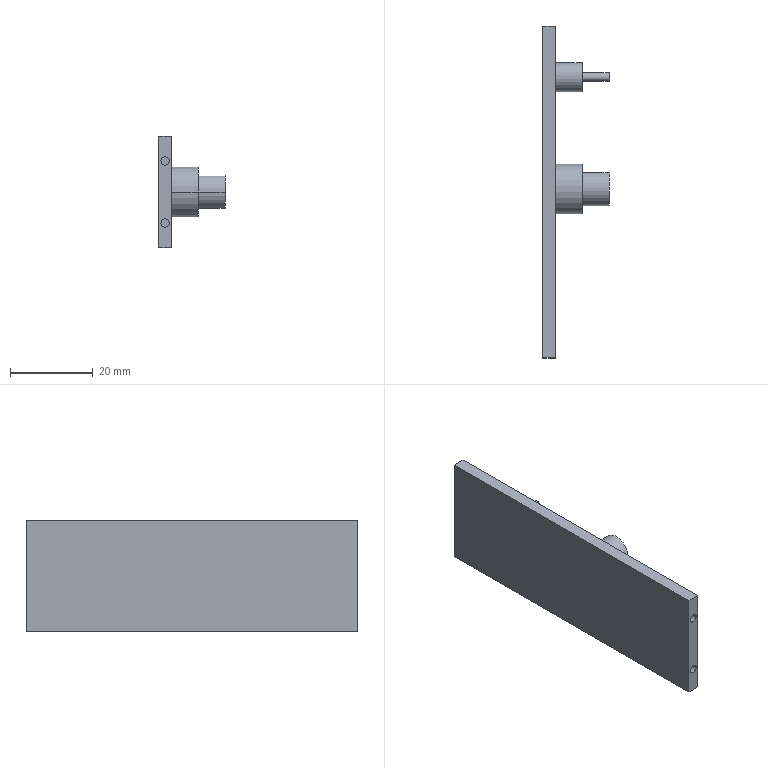Part | SolidWorks | features ICE 2, Cut 1, Extrusion 1 | 1 solid | 24 faces | box 16 x 80 x 27 mm | volume 7781 mm3 | cylinder 12 | plane 12 | commonest cylinder face diameters 2 x6 7 x2 8 x2 12 x2
STEP:
#1=CARTESIAN_POINT('',(-0.4828,4.071,21.));
#2=VERTEX_POINT('',#1);
#3=CARTESIAN_POINT('',(1.517,4.071,21.));
#4=VERTEX_POINT('',#3);
#5=CARTESIAN_POINT('',(0.5172,4.071,21.));
#6=DIRECTION('',(0.,-1.,0.));
#7=DIRECTION('',(1.,0.,0.));
#8=AXIS2_PLACEMENT_3D('',#5,#6,#7);
#9=CIRCLE('',#8,1.);
#10=EDGE_CURVE('',#2,#4,#9,.T.);
#11=ORIENTED_EDGE('',*,*,#10,.F.);
#12=CARTESIAN_POINT('',(-0.4828,-0.9287,21.));
#13=VERTEX_POINT('',#12);
#14=CARTESIAN_POINT('',(-0.4828,4.071,21.));
#15=DIRECTION('',(0.,-1.,0.));
#16=VECTOR('',#15,1000.);
#17=LINE('',#14,#16);
#18=EDGE_CURVE('',#2,#13,#17,.T.);
#19=ORIENTED_EDGE('',*,*,#18,.T.);
#20=CARTESIAN_POINT('',(1.517,-0.9287,21.));
#21=VERTEX_POINT('',#20);
#22=CARTESIAN_POINT('',(0.5172,-0.9287,21.));
#23=DIRECTION('',(0.,1.,0.));
#24=DIRECTION('',(0.,0.,1.));
#25=AXIS2_PLACEMENT_3D('',#22,#23,#24);
#26=CIRCLE('',#25,1.);
#27=EDGE_CURVE('',#21,#13,#26,.T.);
#28=ORIENTED_EDGE('',*,*,#27,.F.);
#29=CARTESIAN_POINT('',(1.517,4.071,21.));
#30=DIRECTION('',(0.,-1.,0.));
#31=VECTOR('',#30,1000.);
#32=LINE('',#29,#31);
#33=EDGE_CURVE('',#4,#21,#32,.T.);
#34=ORIENTED_EDGE('',*,*,#33,.F.);
#35=EDGE_LOOP('',(#11,#19,#28,#34));
#36=FACE_OUTER_BOUND('',#35,.T.);
#37=CARTESIAN_POINT('',(0.5172,4.071,21.));
#38=DIRECTION('',(0.,-1.,0.));
#39=DIRECTION('',(1.,0.,0.));
#40=AXIS2_PLACEMENT_3D('',#37,#38,#39);
#41=CYLINDRICAL_SURFACE('',#40,1.);
#42=ADVANCED_FACE('',(#36),#41,.F.);
#43=CARTESIAN_POINT('',(-0.4828,4.071,6.));
#44=VERTEX_POINT('',#43);
#45=CARTESIAN_POINT('',(1.517,4.071,6.));
#46=VERTEX_POINT('',#45);
#47=CARTESIAN_POINT('',(0.5172,4.071,6.));
#48=DIRECTION('',(0.,-1.,0.));
#49=DIRECTION('',(1.,0.,0.));
#50=AXIS2_PLACEMENT_3D('',#47,#48,#49);
#51=CIRCLE('',#50,1.);
#52=EDGE_CURVE('',#44,#46,#51,.T.);
#53=ORIENTED_EDGE('',*,*,#52,.F.);
#54=CARTESIAN_POINT('',(-0.4828,-0.9287,6.));
#55=VERTEX_POINT('',#54);
#56=CARTESIAN_POINT('',(-0.4828,4.071,6.));
#57=DIRECTION('',(0.,-1.,0.));
#58=VECTOR('',#57,1000.);
#59=LINE('',#56,#58);
#60=EDGE_CURVE('',#44,#55,#59,.T.);
#61=ORIENTED_EDGE('',*,*,#60,.T.);
#62=CARTESIAN_POINT('',(1.517,-0.9287,6.));
#63=VERTEX_POINT('',#62);
#64=CARTESIAN_POINT('',(0.5172,-0.9287,6.));
#65=DIRECTION('',(0.,1.,0.));
#66=DIRECTION('',(0.,0.,1.));
#67=AXIS2_PLACEMENT_3D('',#64,#65,#66);
#68=CIRCLE('',#67,1.);
#69=EDGE_CURVE('',#63,#55,#68,.T.);
#70=ORIENTED_EDGE('',*,*,#69,.F.);
#71=CARTESIAN_POINT('',(1.517,4.071,6.));
#72=DIRECTION('',(0.,-1.,0.));
#73=VECTOR('',#72,1000.);
#74=LINE('',#71,#73);
#75=EDGE_CURVE('',#46,#63,#74,.T.);
#76=ORIENTED_EDGE('',*,*,#75,.F.);
#77=EDGE_LOOP('',(#53,#61,#70,#76));
#78=FACE_OUTER_BOUND('',#77,.T.);
#79=CARTESIAN_POINT('',(0.5172,4.071,6.));
#80=DIRECTION('',(0.,-1.,0.));
#81=DIRECTION('',(1.,0.,0.));
#82=AXIS2_PLACEMENT_3D('',#79,#80,#81);
#83=CYLINDRICAL_SURFACE('',#82,1.);
#84=ADVANCED_FACE('',(#78),#83,.F.);
#85=CARTESIAN_POINT('',(15.017,43.771,13.5));
#86=VERTEX_POINT('',#85);
#87=CARTESIAN_POINT('',(15.017,35.771,13.5));
#88=VERTEX_POINT('',#87);
#89=CARTESIAN_POINT('',(15.017,39.771,13.5));
#90=DIRECTION('',(1.,0.,0.));
#91=DIRECTION('',(0.,1.,0.));
#92=AXIS2_PLACEMENT_3D('',#89,#90,#91);
#93=CIRCLE('',#92,4.);
#94=EDGE_CURVE('',#86,#88,#93,.T.);
#95=ORIENTED_EDGE('',*,*,#94,.F.);
#96=CARTESIAN_POINT('',(8.517,43.771,13.5));
#97=VERTEX_POINT('',#96);
#98=CARTESIAN_POINT('',(15.017,43.771,13.5));
#99=DIRECTION('',(-1.,0.,0.));
#100=VECTOR('',#99,1000.);
#101=LINE('',#98,#100);
#102=EDGE_CURVE('',#86,#97,#101,.T.);
#103=ORIENTED_EDGE('',*,*,#102,.T.);
#104=CARTESIAN_POINT('',(8.517,35.771,13.5));
#105=VERTEX_POINT('',#104);
#106=CARTESIAN_POINT('',(8.517,39.771,13.5));
#107=DIRECTION('',(1.,0.,0.));
#108=DIRECTION('',(0.,1.,0.));
#109=AXIS2_PLACEMENT_3D('',#106,#107,#108);
#110=CIRCLE('',#109,4.);
#111=EDGE_CURVE('',#97,#105,#110,.T.);
#112=ORIENTED_EDGE('',*,*,#111,.T.);
#113=CARTESIAN_POINT('',(15.017,35.771,13.5));
#114=DIRECTION('',(-1.,0.,0.));
#115=VECTOR('',#114,1000.);
#116=LINE('',#113,#115);
#117=EDGE_CURVE('',#88,#105,#116,.T.);
#118=ORIENTED_EDGE('',*,*,#117,.F.);
#119=EDGE_LOOP('',(#95,#103,#112,#118));
#120=FACE_OUTER_BOUND('',#119,.T.);
#121=CARTESIAN_POINT('',(15.017,39.771,13.5));
#122=DIRECTION('',(-1.,0.,0.));
#123=DIRECTION('',(0.,-1.,0.));
#124=AXIS2_PLACEMENT_3D('',#121,#122,#123);
#125=CYLINDRICAL_SURFACE('',#124,4.);
#126=ADVANCED_FACE('',(#120),#125,.T.);
#127=CARTESIAN_POINT('',(15.017,67.771,13.5));
#128=VERTEX_POINT('',#127);
#129=CARTESIAN_POINT('',(15.017,65.771,13.5));
#130=VERTEX_POINT('',#129);
#131=CARTESIAN_POINT('',(15.017,66.771,13.5));
#132=DIRECTION('',(1.,0.,0.));
#133=DIRECTION('',(0.,1.,0.));
#134=AXIS2_PLACEMENT_3D('',#131,#132,#133);
#135=CIRCLE('',#134,1.);
#136=EDGE_CURVE('',#128,#130,#135,.T.);
#137=ORIENTED_EDGE('',*,*,#136,.F.);
#138=CARTESIAN_POINT('',(8.517,67.771,13.5));
#139=VERTEX_POINT('',#138);
#140=CARTESIAN_POINT('',(15.017,67.771,13.5));
#141=DIRECTION('',(-1.,0.,0.));
#142=VECTOR('',#141,1000.);
#143=LINE('',#140,#142);
#144=EDGE_CURVE('',#128,#139,#143,.T.);
#145=ORIENTED_EDGE('',*,*,#144,.T.);
#146=CARTESIAN_POINT('',(8.517,65.771,13.5));
#147=VERTEX_POINT('',#146);
#148=CARTESIAN_POINT('',(8.517,66.771,13.5));
#149=DIRECTION('',(1.,0.,0.));
#150=DIRECTION('',(0.,1.,0.));
#151=AXIS2_PLACEMENT_3D('',#148,#149,#150);
#152=CIRCLE('',#151,1.);
#153=EDGE_CURVE('',#139,#147,#152,.T.);
#154=ORIENTED_EDGE('',*,*,#153,.T.);
#155=CARTESIAN_POINT('',(15.017,65.771,13.5));
#156=DIRECTION('',(-1.,0.,0.));
#157=VECTOR('',#156,1000.);
#158=LINE('',#155,#157);
#159=EDGE_CURVE('',#130,#147,#158,.T.);
#160=ORIENTED_EDGE('',*,*,#159,.F.);
#161=EDGE_LOOP('',(#137,#145,#154,#160));
#162=FACE_OUTER_BOUND('',#161,.T.);
#163=CARTESIAN_POINT('',(15.017,66.771,13.5));
#164=DIRECTION('',(-1.,0.,0.));
#165=DIRECTION('',(0.,-1.,0.));
#166=AXIS2_PLACEMENT_3D('',#163,#164,#165);
#167=CYLINDRICAL_SURFACE('',#166,1.);
#168=ADVANCED_FACE('',(#162),#167,.T.);
#169=CARTESIAN_POINT('',(8.517,70.271,13.5));
#170=VERTEX_POINT('',#169);
#171=CARTESIAN_POINT('',(8.517,63.271,13.5));
#172=VERTEX_POINT('',#171);
#173=CARTESIAN_POINT('',(8.517,66.771,13.5));
#174=DIRECTION('',(1.,0.,0.));
#175=DIRECTION('',(0.,1.,0.));
#176=AXIS2_PLACEMENT_3D('',#173,#174,#175);
#177=CIRCLE('',#176,3.5);
#178=EDGE_CURVE('',#170,#172,#177,.T.);
#179=ORIENTED_EDGE('',*,*,#178,.F.);
#180=CARTESIAN_POINT('',(2.017,70.271,13.5));
#181=VERTEX_POINT('',#180);
#182=CARTESIAN_POINT('',(8.517,70.271,13.5));
#183=DIRECTION('',(-1.,0.,0.));
#184=VECTOR('',#183,1000.);
#185=LINE('',#182,#184);
#186=EDGE_CURVE('',#170,#181,#185,.T.);
#187=ORIENTED_EDGE('',*,*,#186,.T.);
#188=CARTESIAN_POINT('',(2.017,63.271,13.5));
#189=VERTEX_POINT('',#188);
#190=CARTESIAN_POINT('',(2.017,66.771,13.5));
#191=DIRECTION('',(1.,0.,0.));
#192=DIRECTION('',(0.,-1.,0.));
#193=AXIS2_PLACEMENT_3D('',#190,#191,#192);
#194=CIRCLE('',#193,3.5);
#195=EDGE_CURVE('',#181,#189,#194,.T.);
#196=ORIENTED_EDGE('',*,*,#195,.T.);
#197=CARTESIAN_POINT('',(8.517,63.271,13.5));
#198=DIRECTION('',(-1.,0.,0.));
#199=VECTOR('',#198,1000.);
#200=LINE('',#197,#199);
#201=EDGE_CURVE('',#172,#189,#200,.T.);
#202=ORIENTED_EDGE('',*,*,#201,.F.);
#203=EDGE_LOOP('',(#179,#187,#196,#202));
#204=FACE_OUTER_BOUND('',#203,.T.);
#205=CARTESIAN_POINT('',(8.517,66.771,13.5));
#206=DIRECTION('',(-1.,0.,0.));
#207=DIRECTION('',(0.,-1.,0.));
#208=AXIS2_PLACEMENT_3D('',#205,#206,#207);
#209=CYLINDRICAL_SURFACE('',#208,3.5);
#210=ADVANCED_FACE('',(#204),#209,.T.);
#211=CARTESIAN_POINT('',(8.517,45.771,13.5));
#212=VERTEX_POINT('',#211);
#213=CARTESIAN_POINT('',(8.517,33.771,13.5));
#214=VERTEX_POINT('',#213);
#215=CARTESIAN_POINT('',(8.517,39.771,13.5));
#216=DIRECTION('',(1.,0.,0.));
#217=DIRECTION('',(0.,1.,0.));
#218=AXIS2_PLACEMENT_3D('',#215,#216,#217);
#219=CIRCLE('',#218,6.);
#220=EDGE_CURVE('',#212,#214,#219,.T.);
#221=ORIENTED_EDGE('',*,*,#220,.F.);
#222=CARTESIAN_POINT('',(2.017,45.771,13.5));
#223=VERTEX_POINT('',#222);
#224=CARTESIAN_POINT('',(8.517,45.771,13.5));
#225=DIRECTION('',(-1.,0.,0.));
#226=VECTOR('',#225,1000.);
#227=LINE('',#224,#226);
#228=EDGE_CURVE('',#212,#223,#227,.T.);
#229=ORIENTED_EDGE('',*,*,#228,.T.);
#230=CARTESIAN_POINT('',(2.017,33.771,13.5));
#231=VERTEX_POINT('',#230);
#232=CARTESIAN_POINT('',(2.017,39.771,13.5));
#233=DIRECTION('',(1.,0.,0.));
#234=DIRECTION('',(0.,-1.,0.));
#235=AXIS2_PLACEMENT_3D('',#232,#233,#234);
#236=CIRCLE('',#235,6.);
#237=EDGE_CURVE('',#223,#231,#236,.T.);
#238=ORIENTED_EDGE('',*,*,#237,.T.);
#239=CARTESIAN_POINT('',(8.517,33.771,13.5));
#240=DIRECTION('',(-1.,0.,0.));
#241=VECTOR('',#240,1000.);
#242=LINE('',#239,#241);
#243=EDGE_CURVE('',#214,#231,#242,.T.);
#244=ORIENTED_EDGE('',*,*,#243,.F.);
#245=EDGE_LOOP('',(#221,#229,#238,#244));
#246=FACE_OUTER_BOUND('',#245,.T.);
#247=CARTESIAN_POINT('',(8.517,39.771,13.5));
#248=DIRECTION('',(-1.,0.,0.));
#249=DIRECTION('',(0.,-1.,0.));
#250=AXIS2_PLACEMENT_3D('',#247,#248,#249);
#251=CYLINDRICAL_SURFACE('',#250,6.);
#252=ADVANCED_FACE('',(#246),#251,.T.);
#253=CARTESIAN_POINT('',(-0.9828,79.071,0.));
#254=VERTEX_POINT('',#253);
#255=CARTESIAN_POINT('',(-0.9828,-0.9287,0.));
#256=VERTEX_POINT('',#255);
#257=CARTESIAN_POINT('',(-0.9828,79.071,0.));
#258=DIRECTION('',(0.,-1.,0.));
#259=VECTOR('',#258,1000.);
#260=LINE('',#257,#259);
#261=EDGE_CURVE('',#254,#256,#260,.T.);
#262=ORIENTED_EDGE('',*,*,#261,.T.);
#263=CARTESIAN_POINT('',(-0.9828,-0.9287,27.));
#264=VERTEX_POINT('',#263);
#265=CARTESIAN_POINT('',(-0.9828,-0.9287,27.));
#266=DIRECTION('',(0.,0.,-1.));
#267=VECTOR('',#266,1000.);
#268=LINE('',#265,#267);
#269=EDGE_CURVE('',#264,#256,#268,.T.);
#270=ORIENTED_EDGE('',*,*,#269,.F.);
#271=CARTESIAN_POINT('',(-0.9828,79.071,27.));
#272=VERTEX_POINT('',#271);
#273=CARTESIAN_POINT('',(-0.9828,79.071,27.));
#274=DIRECTION('',(0.,-1.,0.));
#275=VECTOR('',#274,1000.);
#276=LINE('',#273,#275);
#277=EDGE_CURVE('',#272,#264,#276,.T.);
#278=ORIENTED_EDGE('',*,*,#277,.F.);
#279=CARTESIAN_POINT('',(-0.9828,79.071,27.));
#280=DIRECTION('',(0.,0.,-1.));
#281=VECTOR('',#280,1000.);
#282=LINE('',#279,#281);
#283=EDGE_CURVE('',#272,#254,#282,.T.);
#284=ORIENTED_EDGE('',*,*,#283,.T.);
#285=EDGE_LOOP('',(#262,#270,#278,#284));
#286=FACE_OUTER_BOUND('',#285,.T.);
#287=CARTESIAN_POINT('',(-0.9828,79.071,27.));
#288=DIRECTION('',(1.,0.,0.));
#289=DIRECTION('',(0.,1.,0.));
#290=AXIS2_PLACEMENT_3D('',#287,#288,#289);
#291=PLANE('',#290);
#292=ADVANCED_FACE('',(#286),#291,.F.);
#293=ORIENTED_EDGE('',*,*,#27,.T.);
#294=CARTESIAN_POINT('',(0.5172,-0.9287,21.));
#295=DIRECTION('',(0.,1.,0.));
#296=DIRECTION('',(0.,0.,1.));
#297=AXIS2_PLACEMENT_3D('',#294,#295,#296);
#298=CIRCLE('',#297,1.);
#299=EDGE_CURVE('',#13,#21,#298,.T.);
#300=ORIENTED_EDGE('',*,*,#299,.T.);
#301=EDGE_LOOP('',(#293,#300));
#302=FACE_BOUND('',#301,.T.);
#303=ORIENTED_EDGE('',*,*,#69,.T.);
#304=CARTESIAN_POINT('',(0.5172,-0.9287,6.));
#305=DIRECTION('',(0.,1.,0.));
#306=DIRECTION('',(0.,0.,1.));
#307=AXIS2_PLACEMENT_3D('',#304,#305,#306);
#308=CIRCLE('',#307,1.);
#309=EDGE_CURVE('',#55,#63,#308,.T.);
#310=ORIENTED_EDGE('',*,*,#309,.T.);
#311=EDGE_LOOP('',(#303,#310));
#312=FACE_BOUND('',#311,.T.);
#313=CARTESIAN_POINT('',(2.017,-0.9287,0.));
#314=VERTEX_POINT('',#313);
#315=CARTESIAN_POINT('',(-0.9828,-0.9287,0.));
#316=DIRECTION('',(1.,0.,0.));
#317=VECTOR('',#316,1000.);
#318=LINE('',#315,#317);
#319=EDGE_CURVE('',#256,#314,#318,.T.);
#320=ORIENTED_EDGE('',*,*,#319,.T.);
#321=CARTESIAN_POINT('',(2.017,-0.9287,27.));
#322=VERTEX_POINT('',#321);
#323=CARTESIAN_POINT('',(2.017,-0.9287,27.));
#324=DIRECTION('',(0.,0.,-1.));
#325=VECTOR('',#324,1000.);
#326=LINE('',#323,#325);
#327=EDGE_CURVE('',#322,#314,#326,.T.);
#328=ORIENTED_EDGE('',*,*,#327,.F.);
#329=CARTESIAN_POINT('',(-0.9828,-0.9287,27.));
#330=DIRECTION('',(1.,0.,0.));
#331=VECTOR('',#330,1000.);
#332=LINE('',#329,#331);
#333=EDGE_CURVE('',#264,#322,#332,.T.);
#334=ORIENTED_EDGE('',*,*,#333,.F.);
#335=ORIENTED_EDGE('',*,*,#269,.T.);
#336=EDGE_LOOP('',(#320,#328,#334,#335));
#337=FACE_OUTER_BOUND('',#336,.T.);
#338=CARTESIAN_POINT('',(-0.9828,-0.9287,27.));
#339=DIRECTION('',(0.,1.,0.));
#340=DIRECTION('',(0.,0.,1.));
#341=AXIS2_PLACEMENT_3D('',#338,#339,#340);
#342=PLANE('',#341);
#343=ADVANCED_FACE('',(#302,#312,#337),#342,.F.);
#344=CARTESIAN_POINT('',(2.017,66.771,13.5));
#345=DIRECTION('',(1.,0.,0.));
#346=DIRECTION('',(0.,-1.,0.));
#347=AXIS2_PLACEMENT_3D('',#344,#345,#346);
#348=CIRCLE('',#347,3.5);
#349=EDGE_CURVE('',#189,#181,#348,.T.);
#350=ORIENTED_EDGE('',*,*,#349,.F.);
#351=ORIENTED_EDGE('',*,*,#195,.F.);
#352=EDGE_LOOP('',(#350,#351));
#353=FACE_BOUND('',#352,.T.);
#354=CARTESIAN_POINT('',(2.017,39.771,13.5));
#355=DIRECTION('',(1.,0.,0.));
#356=DIRECTION('',(0.,-1.,0.));
#357=AXIS2_PLACEMENT_3D('',#354,#355,#356);
#358=CIRCLE('',#357,6.);
#359=EDGE_CURVE('',#231,#223,#358,.T.);
#360=ORIENTED_EDGE('',*,*,#359,.F.);
#361=ORIENTED_EDGE('',*,*,#237,.F.);
#362=EDGE_LOOP('',(#360,#361));
#363=FACE_BOUND('',#362,.T.);
#364=CARTESIAN_POINT('',(2.017,79.071,0.));
#365=VERTEX_POINT('',#364);
#366=CARTESIAN_POINT('',(2.017,79.071,0.));
#367=DIRECTION('',(0.,1.,0.));
#368=VECTOR('',#367,1000.);
#369=LINE('',#366,#368);
#370=EDGE_CURVE('',#314,#365,#369,.T.);
#371=ORIENTED_EDGE('',*,*,#370,.T.);
#372=CARTESIAN_POINT('',(2.017,79.071,27.));
#373=VERTEX_POINT('',#372);
#374=CARTESIAN_POINT('',(2.017,79.071,27.));
#375=DIRECTION('',(0.,0.,-1.));
#376=VECTOR('',#375,1000.);
#377=LINE('',#374,#376);
#378=EDGE_CURVE('',#373,#365,#377,.T.);
#379=ORIENTED_EDGE('',*,*,#378,.F.);
#380=CARTESIAN_POINT('',(2.017,79.071,27.));
#381=DIRECTION('',(0.,1.,0.));
#382=VECTOR('',#381,1000.);
#383=LINE('',#380,#382);
#384=EDGE_CURVE('',#322,#373,#383,.T.);
#385=ORIENTED_EDGE('',*,*,#384,.F.);
#386=ORIENTED_EDGE('',*,*,#327,.T.);
#387=EDGE_LOOP('',(#371,#379,#385,#386));
#388=FACE_OUTER_BOUND('',#387,.T.);
#389=CARTESIAN_POINT('',(2.017,79.071,27.));
#390=DIRECTION('',(-1.,0.,0.));
#391=DIRECTION('',(0.,-1.,0.));
#392=AXIS2_PLACEMENT_3D('',#389,#390,#391);
#393=PLANE('',#392);
#394=ADVANCED_FACE('',(#353,#363,#388),#393,.F.);
#395=CARTESIAN_POINT('',(-0.9828,79.071,0.));
#396=DIRECTION('',(-1.,0.,0.));
#397=VECTOR('',#396,1000.);
#398=LINE('',#395,#397);
#399=EDGE_CURVE('',#365,#254,#398,.T.);
#400=ORIENTED_EDGE('',*,*,#399,.T.);
#401=ORIENTED_EDGE('',*,*,#283,.F.);
#402=CARTESIAN_POINT('',(-0.9828,79.071,27.));
#403=DIRECTION('',(-1.,0.,0.));
#404=VECTOR('',#403,1000.);
#405=LINE('',#402,#404);
#406=EDGE_CURVE('',#373,#272,#405,.T.);
#407=ORIENTED_EDGE('',*,*,#406,.F.);
#408=ORIENTED_EDGE('',*,*,#378,.T.);
#409=EDGE_LOOP('',(#400,#401,#407,#408));
#410=FACE_OUTER_BOUND('',#409,.T.);
#411=CARTESIAN_POINT('',(-0.9828,79.071,27.));
#412=DIRECTION('',(0.,-1.,0.));
#413=DIRECTION('',(0.,0.,-1.));
#414=AXIS2_PLACEMENT_3D('',#411,#412,#413);
#415=PLANE('',#414);
#416=ADVANCED_FACE('',(#410),#415,.F.);
#417=ORIENTED_EDGE('',*,*,#277,.T.);
#418=ORIENTED_EDGE('',*,*,#333,.T.);
#419=ORIENTED_EDGE('',*,*,#384,.T.);
#420=ORIENTED_EDGE('',*,*,#406,.T.);
#421=EDGE_LOOP('',(#417,#418,#419,#420));
#422=FACE_OUTER_BOUND('',#421,.T.);
#423=CARTESIAN_POINT('',(0.,0.,27.));
#424=DIRECTION('',(0.,0.,1.));
#425=DIRECTION('',(1.,0.,0.));
#426=AXIS2_PLACEMENT_3D('',#423,#424,#425);
#427=PLANE('',#426);
#428=ADVANCED_FACE('',(#422),#427,.T.);
#429=ORIENTED_EDGE('',*,*,#261,.F.);
#430=ORIENTED_EDGE('',*,*,#399,.F.);
#431=ORIENTED_EDGE('',*,*,#370,.F.);
#432=ORIENTED_EDGE('',*,*,#319,.F.);
#433=EDGE_LOOP('',(#429,#430,#431,#432));
#434=FACE_OUTER_BOUND('',#433,.T.);
#435=CARTESIAN_POINT('',(0.,0.,0.));
#436=DIRECTION('',(0.,0.,1.));
#437=DIRECTION('',(1.,0.,0.));
#438=AXIS2_PLACEMENT_3D('',#435,#436,#437);
#439=PLANE('',#438);
#440=ADVANCED_FACE('',(#434),#439,.F.);
#441=ORIENTED_EDGE('',*,*,#228,.F.);
#442=CARTESIAN_POINT('',(8.517,39.771,13.5));
#443=DIRECTION('',(1.,0.,0.));
#444=DIRECTION('',(0.,1.,0.));
#445=AXIS2_PLACEMENT_3D('',#442,#443,#444);
#446=CIRCLE('',#445,6.);
#447=EDGE_CURVE('',#214,#212,#446,.T.);
#448=ORIENTED_EDGE('',*,*,#447,.F.);
#449=ORIENTED_EDGE('',*,*,#243,.T.);
#450=ORIENTED_EDGE('',*,*,#359,.T.);
#451=EDGE_LOOP('',(#441,#448,#449,#450));
#452=FACE_OUTER_BOUND('',#451,.T.);
#453=CARTESIAN_POINT('',(8.517,39.771,13.5));
#454=DIRECTION('',(-1.,0.,0.));
#455=DIRECTION('',(0.,-1.,0.));
#456=AXIS2_PLACEMENT_3D('',#453,#454,#455);
#457=CYLINDRICAL_SURFACE('',#456,6.);
#458=ADVANCED_FACE('',(#452),#457,.T.);
#459=CARTESIAN_POINT('',(8.517,39.771,13.5));
#460=DIRECTION('',(1.,0.,0.));
#461=DIRECTION('',(0.,1.,0.));
#462=AXIS2_PLACEMENT_3D('',#459,#460,#461);
#463=CIRCLE('',#462,4.);
#464=EDGE_CURVE('',#105,#97,#463,.T.);
#465=ORIENTED_EDGE('',*,*,#464,.F.);
#466=ORIENTED_EDGE('',*,*,#111,.F.);
#467=EDGE_LOOP('',(#465,#466));
#468=FACE_BOUND('',#467,.T.);
#469=ORIENTED_EDGE('',*,*,#447,.T.);
#470=ORIENTED_EDGE('',*,*,#220,.T.);
#471=EDGE_LOOP('',(#469,#470));
#472=FACE_OUTER_BOUND('',#471,.T.);
#473=CARTESIAN_POINT('',(8.517,39.771,13.5));
#474=DIRECTION('',(1.,0.,0.));
#475=DIRECTION('',(0.,1.,0.));
#476=AXIS2_PLACEMENT_3D('',#473,#474,#475);
#477=PLANE('',#476);
#478=ADVANCED_FACE('',(#468,#472),#477,.T.);
#479=ORIENTED_EDGE('',*,*,#186,.F.);
#480=CARTESIAN_POINT('',(8.517,66.771,13.5));
#481=DIRECTION('',(1.,0.,0.));
#482=DIRECTION('',(0.,1.,0.));
#483=AXIS2_PLACEMENT_3D('',#480,#481,#482);
#484=CIRCLE('',#483,3.5);
#485=EDGE_CURVE('',#172,#170,#484,.T.);
#486=ORIENTED_EDGE('',*,*,#485,.F.);
#487=ORIENTED_EDGE('',*,*,#201,.T.);
#488=ORIENTED_EDGE('',*,*,#349,.T.);
#489=EDGE_LOOP('',(#479,#486,#487,#488));
#490=FACE_OUTER_BOUND('',#489,.T.);
#491=CARTESIAN_POINT('',(8.517,66.771,13.5));
#492=DIRECTION('',(-1.,0.,0.));
#493=DIRECTION('',(0.,-1.,0.));
#494=AXIS2_PLACEMENT_3D('',#491,#492,#493);
#495=CYLINDRICAL_SURFACE('',#494,3.5);
#496=ADVANCED_FACE('',(#490),#495,.T.);
#497=CARTESIAN_POINT('',(8.517,66.771,13.5));
#498=DIRECTION('',(1.,0.,0.));
#499=DIRECTION('',(0.,1.,0.));
#500=AXIS2_PLACEMENT_3D('',#497,#498,#499);
#501=CIRCLE('',#500,1.);
#502=EDGE_CURVE('',#147,#139,#501,.T.);
#503=ORIENTED_EDGE('',*,*,#502,.F.);
#504=ORIENTED_EDGE('',*,*,#153,.F.);
#505=EDGE_LOOP('',(#503,#504));
#506=FACE_BOUND('',#505,.T.);
#507=ORIENTED_EDGE('',*,*,#485,.T.);
#508=ORIENTED_EDGE('',*,*,#178,.T.);
#509=EDGE_LOOP('',(#507,#508));
#510=FACE_OUTER_BOUND('',#509,.T.);
#511=CARTESIAN_POINT('',(8.517,66.771,13.5));
#512=DIRECTION('',(1.,0.,0.));
#513=DIRECTION('',(0.,1.,0.));
#514=AXIS2_PLACEMENT_3D('',#511,#512,#513);
#515=PLANE('',#514);
#516=ADVANCED_FACE('',(#506,#510),#515,.T.);
#517=ORIENTED_EDGE('',*,*,#144,.F.);
#518=CARTESIAN_POINT('',(15.017,66.771,13.5));
#519=DIRECTION('',(1.,0.,0.));
#520=DIRECTION('',(0.,1.,0.));
#521=AXIS2_PLACEMENT_3D('',#518,#519,#520);
#522=CIRCLE('',#521,1.);
#523=EDGE_CURVE('',#130,#128,#522,.T.);
#524=ORIENTED_EDGE('',*,*,#523,.F.);
#525=ORIENTED_EDGE('',*,*,#159,.T.);
#526=ORIENTED_EDGE('',*,*,#502,.T.);
#527=EDGE_LOOP('',(#517,#524,#525,#526));
#528=FACE_OUTER_BOUND('',#527,.T.);
#529=CARTESIAN_POINT('',(15.017,66.771,13.5));
#530=DIRECTION('',(-1.,0.,0.));
#531=DIRECTION('',(0.,-1.,0.));
#532=AXIS2_PLACEMENT_3D('',#529,#530,#531);
#533=CYLINDRICAL_SURFACE('',#532,1.);
#534=ADVANCED_FACE('',(#528),#533,.T.);
#535=ORIENTED_EDGE('',*,*,#523,.T.);
#536=ORIENTED_EDGE('',*,*,#136,.T.);
#537=EDGE_LOOP('',(#535,#536));
#538=FACE_OUTER_BOUND('',#537,.T.);
#539=CARTESIAN_POINT('',(15.017,66.771,13.5));
#540=DIRECTION('',(1.,0.,0.));
#541=DIRECTION('',(0.,1.,0.));
#542=AXIS2_PLACEMENT_3D('',#539,#540,#541);
#543=PLANE('',#542);
#544=ADVANCED_FACE('',(#538),#543,.T.);
#545=ORIENTED_EDGE('',*,*,#102,.F.);
#546=CARTESIAN_POINT('',(15.017,39.771,13.5));
#547=DIRECTION('',(1.,0.,0.));
#548=DIRECTION('',(0.,1.,0.));
#549=AXIS2_PLACEMENT_3D('',#546,#547,#548);
#550=CIRCLE('',#549,4.);
#551=EDGE_CURVE('',#88,#86,#550,.T.);
#552=ORIENTED_EDGE('',*,*,#551,.F.);
#553=ORIENTED_EDGE('',*,*,#117,.T.);
#554=ORIENTED_EDGE('',*,*,#464,.T.);
#555=EDGE_LOOP('',(#545,#552,#553,#554));
#556=FACE_OUTER_BOUND('',#555,.T.);
#557=CARTESIAN_POINT('',(15.017,39.771,13.5));
#558=DIRECTION('',(-1.,0.,0.));
#559=DIRECTION('',(0.,-1.,0.));
#560=AXIS2_PLACEMENT_3D('',#557,#558,#559);
#561=CYLINDRICAL_SURFACE('',#560,4.);
#562=ADVANCED_FACE('',(#556),#561,.T.);
#563=ORIENTED_EDGE('',*,*,#551,.T.);
#564=ORIENTED_EDGE('',*,*,#94,.T.);
#565=EDGE_LOOP('',(#563,#564));
#566=FACE_OUTER_BOUND('',#565,.T.);
#567=CARTESIAN_POINT('',(15.017,39.771,13.5));
#568=DIRECTION('',(1.,0.,0.));
#569=DIRECTION('',(0.,1.,0.));
#570=AXIS2_PLACEMENT_3D('',#567,#568,#569);
#571=PLANE('',#570);
#572=ADVANCED_FACE('',(#566),#571,.T.);
#573=ORIENTED_EDGE('',*,*,#60,.F.);
#574=CARTESIAN_POINT('',(0.5172,4.071,6.));
#575=DIRECTION('',(0.,-1.,0.));
#576=DIRECTION('',(1.,0.,0.));
#577=AXIS2_PLACEMENT_3D('',#574,#575,#576);
#578=CIRCLE('',#577,1.);
#579=EDGE_CURVE('',#46,#44,#578,.T.);
#580=ORIENTED_EDGE('',*,*,#579,.F.);
#581=ORIENTED_EDGE('',*,*,#75,.T.);
#582=ORIENTED_EDGE('',*,*,#309,.F.);
#583=EDGE_LOOP('',(#573,#580,#581,#582));
#584=FACE_OUTER_BOUND('',#583,.T.);
#585=CARTESIAN_POINT('',(0.5172,4.071,6.));
#586=DIRECTION('',(0.,-1.,0.));
#587=DIRECTION('',(1.,0.,0.));
#588=AXIS2_PLACEMENT_3D('',#585,#586,#587);
#589=CYLINDRICAL_SURFACE('',#588,1.);
#590=ADVANCED_FACE('',(#584),#589,.F.);
#591=ORIENTED_EDGE('',*,*,#579,.T.);
#592=ORIENTED_EDGE('',*,*,#52,.T.);
#593=EDGE_LOOP('',(#591,#592));
#594=FACE_OUTER_BOUND('',#593,.T.);
#595=CARTESIAN_POINT('',(0.5172,4.071,6.));
#596=DIRECTION('',(0.,-1.,0.));
#597=DIRECTION('',(1.,0.,0.));
#598=AXIS2_PLACEMENT_3D('',#595,#596,#597);
#599=PLANE('',#598);
#600=ADVANCED_FACE('',(#594),#599,.T.);
#601=ORIENTED_EDGE('',*,*,#18,.F.);
#602=CARTESIAN_POINT('',(0.5172,4.071,21.));
#603=DIRECTION('',(0.,-1.,0.));
#604=DIRECTION('',(1.,0.,0.));
#605=AXIS2_PLACEMENT_3D('',#602,#603,#604);
#606=CIRCLE('',#605,1.);
#607=EDGE_CURVE('',#4,#2,#606,.T.);
#608=ORIENTED_EDGE('',*,*,#607,.F.);
#609=ORIENTED_EDGE('',*,*,#33,.T.);
#610=ORIENTED_EDGE('',*,*,#299,.F.);
#611=EDGE_LOOP('',(#601,#608,#609,#610));
#612=FACE_OUTER_BOUND('',#611,.T.);
#613=CARTESIAN_POINT('',(0.5172,4.071,21.));
#614=DIRECTION('',(0.,-1.,0.));
#615=DIRECTION('',(1.,0.,0.));
#616=AXIS2_PLACEMENT_3D('',#613,#614,#615);
#617=CYLINDRICAL_SURFACE('',#616,1.);
#618=ADVANCED_FACE('',(#612),#617,.F.);
#619=ORIENTED_EDGE('',*,*,#607,.T.);
#620=ORIENTED_EDGE('',*,*,#10,.T.);
#621=EDGE_LOOP('',(#619,#620));
#622=FACE_OUTER_BOUND('',#621,.T.);
#623=CARTESIAN_POINT('',(0.5172,4.071,21.));
#624=DIRECTION('',(0.,-1.,0.));
#625=DIRECTION('',(1.,0.,0.));
#626=AXIS2_PLACEMENT_3D('',#623,#624,#625);
#627=PLANE('',#626);
#628=ADVANCED_FACE('',(#622),#627,.T.);
#629=CLOSED_SHELL('',(#42,#84,#126,#168,#210,#252,#292,#343,#394,#416,#428,#440,#458,#478,#496,#516,#534,#544,#562,#572,#590,#600,#618,#628));
#630=MANIFOLD_SOLID_BREP('',#629);
#631=CARTESIAN_POINT('',(0.,0.,0.));
#632=DIRECTION('',(0.,0.,1.));
#633=DIRECTION('',(1.,0.,0.));
#634=AXIS2_PLACEMENT_3D('',#631,#632,#633);
#635=(LENGTH_UNIT()NAMED_UNIT(*)SI_UNIT(.MILLI.,.METRE.));
#636=UNCERTAINTY_MEASURE_WITH_UNIT(LENGTH_MEASURE(0.00001),#635,'','');
#637=(NAMED_UNIT(*)PLANE_ANGLE_UNIT()SI_UNIT($,.RADIAN.));
#638=(NAMED_UNIT(*)SI_UNIT($,.STERADIAN.)SOLID_ANGLE_UNIT());
#639=(GEOMETRIC_REPRESENTATION_CONTEXT(3)GLOBAL_UNCERTAINTY_ASSIGNED_CONTEXT((#636))GLOBAL_UNIT_ASSIGNED_CONTEXT((#635,#637,#638))REPRESENTATION_CONTEXT('',''));
#640=ADVANCED_BREP_SHAPE_REPRESENTATION('',(#630,#634),#639);